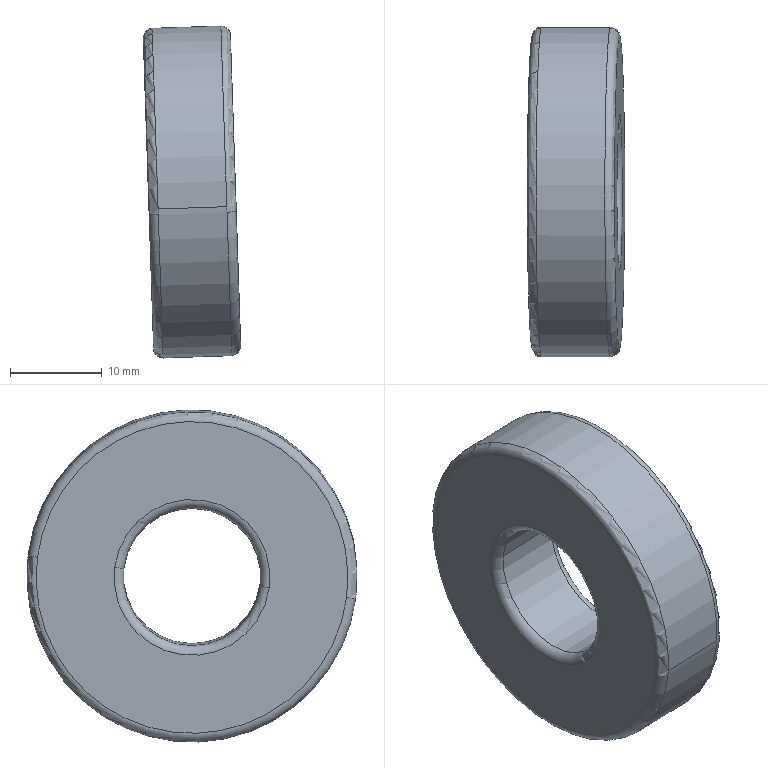Part | STEP file | 2026.6.15-Main Assembly图.sldasm-Part-94 | 1 solid | 14 faces | box 10.629 x 36.003 x 36.231 mm | volume 7922 mm3 | torus 8 | cylinder 4 | plane 2 | commonest cylinder face diameters 15 x2 36 x2
STEP:
#1=CARTESIAN_POINT('',(-1546.876,1321.722,3701.345));
#2=VERTEX_POINT('',#1);
#3=CARTESIAN_POINT('',(-1546.997,1357.487,3705.403));
#4=VERTEX_POINT('',#3);
#5=CARTESIAN_POINT('',(-1546.947,1339.57,3703.676));
#6=DIRECTION('',(0.9994,-0.0004028,0.03334));
#7=DIRECTION('',(-0.003921,0.9916,0.1295));
#8=AXIS2_PLACEMENT_3D('',#5,#6,#7);
#9=CIRCLE('',#8,18.);
#10=EDGE_CURVE('',#2,#4,#9,.T.);
#11=ORIENTED_EDGE('',*,*,#10,.F.);
#12=CARTESIAN_POINT('',(-1547.88,1322.714,3701.441));
#13=VERTEX_POINT('',#12);
#14=CARTESIAN_POINT('',(-1546.88,1322.713,3701.474));
#15=DIRECTION('',(0.03311,0.1296,-0.991));
#16=DIRECTION('',(0.,0.9916,0.1297));
#17=AXIS2_PLACEMENT_3D('',#14,#15,#16);
#18=CIRCLE('',#17,1.);
#19=EDGE_CURVE('',#2,#13,#18,.T.);
#20=ORIENTED_EDGE('',*,*,#19,.T.);
#21=CARTESIAN_POINT('',(-1548.013,1356.427,3705.845));
#22=VERTEX_POINT('',#21);
#23=CARTESIAN_POINT('',(-1547.946,1339.57,3703.643));
#24=DIRECTION('',(-0.9994,0.0004028,-0.03334));
#25=DIRECTION('',(-0.003921,0.9916,0.1295));
#26=AXIS2_PLACEMENT_3D('',#23,#24,#25);
#27=CIRCLE('',#26,17.);
#28=EDGE_CURVE('',#22,#13,#27,.T.);
#29=ORIENTED_EDGE('',*,*,#28,.F.);
#30=CARTESIAN_POINT('',(-1547.017,1357.418,3706.008));
#31=VERTEX_POINT('',#30);
#32=CARTESIAN_POINT('',(-1547.014,1356.427,3705.878));
#33=DIRECTION('',(-0.03311,-0.1296,0.991));
#34=DIRECTION('',(0.,-0.9916,-0.1297));
#35=AXIS2_PLACEMENT_3D('',#32,#33,#34);
#36=CIRCLE('',#35,1.);
#37=EDGE_CURVE('',#31,#22,#36,.T.);
#38=ORIENTED_EDGE('',*,*,#37,.F.);
#39=CARTESIAN_POINT('',(-1546.947,1339.57,3703.676));
#40=DIRECTION('',(0.9994,-0.0004028,0.03334));
#41=DIRECTION('',(-0.003921,0.9916,0.1295));
#42=AXIS2_PLACEMENT_3D('',#39,#40,#41);
#43=CIRCLE('',#42,18.);
#44=EDGE_CURVE('',#4,#31,#43,.T.);
#45=ORIENTED_EDGE('',*,*,#44,.F.);
#46=EDGE_LOOP('',(#11,#20,#29,#38,#45));
#47=FACE_OUTER_BOUND('',#46,.T.);
#48=CARTESIAN_POINT('',(-1546.947,1339.57,3703.676));
#49=DIRECTION('',(-0.9994,0.0004028,-0.03334));
#50=DIRECTION('',(-0.003921,0.9916,0.1295));
#51=AXIS2_PLACEMENT_3D('',#48,#49,#50);
#52=TOROIDAL_SURFACE('',#51,17.,1.);
#53=ADVANCED_FACE('',(#47),#52,.T.);
#54=CARTESIAN_POINT('',(-1547.913,1331.142,3702.542));
#55=VERTEX_POINT('',#54);
#56=CARTESIAN_POINT('',(-1547.98,1347.999,3704.744));
#57=VERTEX_POINT('',#56);
#58=CARTESIAN_POINT('',(-1547.946,1339.57,3703.643));
#59=DIRECTION('',(0.9994,-0.0004028,0.03334));
#60=DIRECTION('',(-0.003921,0.9916,0.1295));
#61=AXIS2_PLACEMENT_3D('',#58,#59,#60);
#62=CIRCLE('',#61,8.5);
#63=EDGE_CURVE('',#55,#57,#62,.T.);
#64=ORIENTED_EDGE('',*,*,#63,.F.);
#65=CARTESIAN_POINT('',(-1546.917,1332.133,3702.705));
#66=VERTEX_POINT('',#65);
#67=CARTESIAN_POINT('',(-1546.914,1331.142,3702.575));
#68=DIRECTION('',(0.03311,0.1296,-0.991));
#69=DIRECTION('',(0.,0.9916,0.1297));
#70=AXIS2_PLACEMENT_3D('',#67,#68,#69);
#71=CIRCLE('',#70,1.);
#72=EDGE_CURVE('',#55,#66,#71,.T.);
#73=ORIENTED_EDGE('',*,*,#72,.T.);
#74=CARTESIAN_POINT('',(-1546.976,1347.007,3704.648));
#75=VERTEX_POINT('',#74);
#76=CARTESIAN_POINT('',(-1546.947,1339.57,3703.676));
#77=DIRECTION('',(-0.9994,0.0004028,-0.03334));
#78=DIRECTION('',(-0.003921,0.9916,0.1295));
#79=AXIS2_PLACEMENT_3D('',#76,#77,#78);
#80=CIRCLE('',#79,7.5);
#81=EDGE_CURVE('',#75,#66,#80,.T.);
#82=ORIENTED_EDGE('',*,*,#81,.F.);
#83=CARTESIAN_POINT('',(-1546.98,1347.998,3704.777));
#84=DIRECTION('',(-0.03311,-0.1296,0.991));
#85=DIRECTION('',(0.,-0.9916,-0.1297));
#86=AXIS2_PLACEMENT_3D('',#83,#84,#85);
#87=CIRCLE('',#86,1.);
#88=EDGE_CURVE('',#57,#75,#87,.T.);
#89=ORIENTED_EDGE('',*,*,#88,.F.);
#90=EDGE_LOOP('',(#64,#73,#82,#89));
#91=FACE_OUTER_BOUND('',#90,.T.);
#92=CARTESIAN_POINT('',(-1546.947,1339.57,3703.676));
#93=DIRECTION('',(-0.9994,0.0004028,-0.03334));
#94=DIRECTION('',(-0.003921,0.9916,0.1295));
#95=AXIS2_PLACEMENT_3D('',#92,#93,#94);
#96=TOROIDAL_SURFACE('',#95,8.5,1.);
#97=ADVANCED_FACE('',(#91),#96,.T.);
#98=CARTESIAN_POINT('',(-1538.485,1347.995,3705.061));
#99=VERTEX_POINT('',#98);
#100=CARTESIAN_POINT('',(-1538.418,1331.138,3702.859));
#101=VERTEX_POINT('',#100);
#102=CARTESIAN_POINT('',(-1538.452,1339.567,3703.96));
#103=DIRECTION('',(-0.9994,0.0004028,-0.03334));
#104=DIRECTION('',(0.003921,-0.9916,-0.1295));
#105=AXIS2_PLACEMENT_3D('',#102,#103,#104);
#106=CIRCLE('',#105,8.5);
#107=EDGE_CURVE('',#99,#101,#106,.T.);
#108=ORIENTED_EDGE('',*,*,#107,.F.);
#109=CARTESIAN_POINT('',(-1539.48,1347.004,3704.898));
#110=VERTEX_POINT('',#109);
#111=CARTESIAN_POINT('',(-1539.484,1347.995,3705.027));
#112=DIRECTION('',(0.03311,0.1296,-0.991));
#113=DIRECTION('',(0.,0.9916,0.1297));
#114=AXIS2_PLACEMENT_3D('',#111,#112,#113);
#115=CIRCLE('',#114,1.);
#116=EDGE_CURVE('',#99,#110,#115,.T.);
#117=ORIENTED_EDGE('',*,*,#116,.T.);
#118=CARTESIAN_POINT('',(-1539.422,1332.13,3702.955));
#119=VERTEX_POINT('',#118);
#120=CARTESIAN_POINT('',(-1539.451,1339.567,3703.926));
#121=DIRECTION('',(0.9994,-0.0004028,0.03334));
#122=DIRECTION('',(0.003921,-0.9916,-0.1295));
#123=AXIS2_PLACEMENT_3D('',#120,#121,#122);
#124=CIRCLE('',#123,7.5);
#125=EDGE_CURVE('',#119,#110,#124,.T.);
#126=ORIENTED_EDGE('',*,*,#125,.F.);
#127=CARTESIAN_POINT('',(-1539.418,1331.139,3702.825));
#128=DIRECTION('',(-0.03311,-0.1296,0.991));
#129=DIRECTION('',(0.,-0.9916,-0.1297));
#130=AXIS2_PLACEMENT_3D('',#127,#128,#129);
#131=CIRCLE('',#130,1.);
#132=EDGE_CURVE('',#101,#119,#131,.T.);
#133=ORIENTED_EDGE('',*,*,#132,.F.);
#134=EDGE_LOOP('',(#108,#117,#126,#133));
#135=FACE_OUTER_BOUND('',#134,.T.);
#136=CARTESIAN_POINT('',(-1539.451,1339.567,3703.926));
#137=DIRECTION('',(0.9994,-0.0004028,0.03334));
#138=DIRECTION('',(0.003921,-0.9916,-0.1295));
#139=AXIS2_PLACEMENT_3D('',#136,#137,#138);
#140=TOROIDAL_SURFACE('',#139,8.5,1.);
#141=ADVANCED_FACE('',(#135),#140,.T.);
#142=CARTESIAN_POINT('',(-1539.522,1357.415,3706.258));
#143=VERTEX_POINT('',#142);
#144=CARTESIAN_POINT('',(-1539.501,1357.484,3705.653));
#145=VERTEX_POINT('',#144);
#146=CARTESIAN_POINT('',(-1539.451,1339.567,3703.926));
#147=DIRECTION('',(-0.9994,0.0004028,-0.03334));
#148=DIRECTION('',(0.003921,-0.9916,-0.1295));
#149=AXIS2_PLACEMENT_3D('',#146,#147,#148);
#150=CIRCLE('',#149,18.);
#151=EDGE_CURVE('',#143,#145,#150,.T.);
#152=ORIENTED_EDGE('',*,*,#151,.F.);
#153=CARTESIAN_POINT('',(-1538.518,1356.423,3706.162));
#154=VERTEX_POINT('',#153);
#155=CARTESIAN_POINT('',(-1539.518,1356.424,3706.128));
#156=DIRECTION('',(0.03311,0.1296,-0.991));
#157=DIRECTION('',(0.,0.9916,0.1297));
#158=AXIS2_PLACEMENT_3D('',#155,#156,#157);
#159=CIRCLE('',#158,1.);
#160=EDGE_CURVE('',#143,#154,#159,.T.);
#161=ORIENTED_EDGE('',*,*,#160,.T.);
#162=CARTESIAN_POINT('',(-1538.385,1322.71,3701.758));
#163=VERTEX_POINT('',#162);
#164=CARTESIAN_POINT('',(-1538.452,1339.567,3703.96));
#165=DIRECTION('',(0.9994,-0.0004028,0.03334));
#166=DIRECTION('',(0.003921,-0.9916,-0.1295));
#167=AXIS2_PLACEMENT_3D('',#164,#165,#166);
#168=CIRCLE('',#167,17.);
#169=EDGE_CURVE('',#163,#154,#168,.T.);
#170=ORIENTED_EDGE('',*,*,#169,.F.);
#171=CARTESIAN_POINT('',(-1539.38,1321.719,3701.595));
#172=VERTEX_POINT('',#171);
#173=CARTESIAN_POINT('',(-1539.384,1322.71,3701.724));
#174=DIRECTION('',(-0.03311,-0.1296,0.991));
#175=DIRECTION('',(0.,-0.9916,-0.1297));
#176=AXIS2_PLACEMENT_3D('',#173,#174,#175);
#177=CIRCLE('',#176,1.);
#178=EDGE_CURVE('',#172,#163,#177,.T.);
#179=ORIENTED_EDGE('',*,*,#178,.F.);
#180=CARTESIAN_POINT('',(-1539.451,1339.567,3703.926));
#181=DIRECTION('',(-0.9994,0.0004028,-0.03334));
#182=DIRECTION('',(0.003921,-0.9916,-0.1295));
#183=AXIS2_PLACEMENT_3D('',#180,#181,#182);
#184=CIRCLE('',#183,18.);
#185=EDGE_CURVE('',#145,#172,#184,.T.);
#186=ORIENTED_EDGE('',*,*,#185,.F.);
#187=EDGE_LOOP('',(#152,#161,#170,#179,#186));
#188=FACE_OUTER_BOUND('',#187,.T.);
#189=CARTESIAN_POINT('',(-1539.451,1339.567,3703.926));
#190=DIRECTION('',(0.9994,-0.0004028,0.03334));
#191=DIRECTION('',(0.003921,-0.9916,-0.1295));
#192=AXIS2_PLACEMENT_3D('',#189,#190,#191);
#193=TOROIDAL_SURFACE('',#192,17.,1.);
#194=ADVANCED_FACE('',(#188),#193,.T.);
#195=CARTESIAN_POINT('',(-1546.947,1339.57,3703.676));
#196=DIRECTION('',(-0.9994,0.0004028,-0.03334));
#197=DIRECTION('',(-0.003921,0.9916,0.1295));
#198=AXIS2_PLACEMENT_3D('',#195,#196,#197);
#199=CIRCLE('',#198,7.5);
#200=EDGE_CURVE('',#66,#75,#199,.T.);
#201=ORIENTED_EDGE('',*,*,#200,.T.);
#202=CARTESIAN_POINT('',(-1547.976,1347.007,3704.614));
#203=DIRECTION('',(0.9994,-0.0004028,0.03334));
#204=VECTOR('',#203,1000.);
#205=LINE('',#202,#204);
#206=EDGE_CURVE('',#75,#110,#205,.T.);
#207=ORIENTED_EDGE('',*,*,#206,.T.);
#208=CARTESIAN_POINT('',(-1539.451,1339.567,3703.926));
#209=DIRECTION('',(0.9994,-0.0004028,0.03334));
#210=DIRECTION('',(0.003921,-0.9916,-0.1295));
#211=AXIS2_PLACEMENT_3D('',#208,#209,#210);
#212=CIRCLE('',#211,7.5);
#213=EDGE_CURVE('',#110,#119,#212,.T.);
#214=ORIENTED_EDGE('',*,*,#213,.T.);
#215=CARTESIAN_POINT('',(-1547.917,1332.134,3702.671));
#216=DIRECTION('',(0.9994,-0.0004028,0.03334));
#217=VECTOR('',#216,1000.);
#218=LINE('',#215,#217);
#219=EDGE_CURVE('',#66,#119,#218,.T.);
#220=ORIENTED_EDGE('',*,*,#219,.F.);
#221=EDGE_LOOP('',(#201,#207,#214,#220));
#222=FACE_OUTER_BOUND('',#221,.T.);
#223=CARTESIAN_POINT('',(-1547.946,1339.57,3703.643));
#224=DIRECTION('',(0.9994,-0.0004028,0.03334));
#225=DIRECTION('',(0.003921,-0.9916,-0.1295));
#226=AXIS2_PLACEMENT_3D('',#223,#224,#225);
#227=CYLINDRICAL_SURFACE('',#226,7.5);
#228=ADVANCED_FACE('',(#222),#227,.F.);
#229=ORIENTED_EDGE('',*,*,#44,.T.);
#230=CARTESIAN_POINT('',(-1546.896,1321.653,3701.949));
#231=VERTEX_POINT('',#230);
#232=CARTESIAN_POINT('',(-1546.947,1339.57,3703.676));
#233=DIRECTION('',(0.9994,-0.0004028,0.03334));
#234=DIRECTION('',(-0.003921,0.9916,0.1295));
#235=AXIS2_PLACEMENT_3D('',#232,#233,#234);
#236=CIRCLE('',#235,18.);
#237=EDGE_CURVE('',#31,#231,#236,.T.);
#238=ORIENTED_EDGE('',*,*,#237,.T.);
#239=CARTESIAN_POINT('',(-1539.401,1321.65,3702.199));
#240=VERTEX_POINT('',#239);
#241=CARTESIAN_POINT('',(-1547.896,1321.653,3701.916));
#242=DIRECTION('',(0.9994,-0.0004028,0.03334));
#243=VECTOR('',#242,1000.);
#244=LINE('',#241,#243);
#245=EDGE_CURVE('',#231,#240,#244,.T.);
#246=ORIENTED_EDGE('',*,*,#245,.T.);
#247=CARTESIAN_POINT('',(-1539.451,1339.567,3703.926));
#248=DIRECTION('',(-0.9994,0.0004028,-0.03334));
#249=DIRECTION('',(0.003921,-0.9916,-0.1295));
#250=AXIS2_PLACEMENT_3D('',#247,#248,#249);
#251=CIRCLE('',#250,18.);
#252=EDGE_CURVE('',#240,#143,#251,.T.);
#253=ORIENTED_EDGE('',*,*,#252,.T.);
#254=ORIENTED_EDGE('',*,*,#151,.T.);
#255=CARTESIAN_POINT('',(-1547.997,1357.487,3705.37));
#256=DIRECTION('',(0.9994,-0.0004028,0.03334));
#257=VECTOR('',#256,1000.);
#258=LINE('',#255,#257);
#259=EDGE_CURVE('',#4,#145,#258,.T.);
#260=ORIENTED_EDGE('',*,*,#259,.F.);
#261=EDGE_LOOP('',(#229,#238,#246,#253,#254,#260));
#262=FACE_OUTER_BOUND('',#261,.T.);
#263=CARTESIAN_POINT('',(-1547.946,1339.57,3703.643));
#264=DIRECTION('',(0.9994,-0.0004028,0.03334));
#265=DIRECTION('',(-0.002799,0.9954,0.09594));
#266=AXIS2_PLACEMENT_3D('',#263,#264,#265);
#267=CYLINDRICAL_SURFACE('',#266,18.);
#268=ADVANCED_FACE('',(#262),#267,.T.);
#269=ORIENTED_EDGE('',*,*,#169,.T.);
#270=CARTESIAN_POINT('',(-1538.452,1339.567,3703.96));
#271=DIRECTION('',(0.9994,-0.0004028,0.03334));
#272=DIRECTION('',(0.003921,-0.9916,-0.1295));
#273=AXIS2_PLACEMENT_3D('',#270,#271,#272);
#274=CIRCLE('',#273,17.);
#275=EDGE_CURVE('',#154,#163,#274,.T.);
#276=ORIENTED_EDGE('',*,*,#275,.T.);
#277=EDGE_LOOP('',(#269,#276));
#278=FACE_OUTER_BOUND('',#277,.T.);
#279=CARTESIAN_POINT('',(-1538.452,1339.567,3703.96));
#280=DIRECTION('',(-0.9994,0.0004028,-0.03334));
#281=DIRECTION('',(0.003921,-0.9916,-0.1295));
#282=AXIS2_PLACEMENT_3D('',#279,#280,#281);
#283=CIRCLE('',#282,8.5);
#284=EDGE_CURVE('',#101,#99,#283,.T.);
#285=ORIENTED_EDGE('',*,*,#284,.T.);
#286=ORIENTED_EDGE('',*,*,#107,.T.);
#287=EDGE_LOOP('',(#285,#286));
#288=FACE_BOUND('',#287,.T.);
#289=CARTESIAN_POINT('',(-1538.452,1339.567,3703.96));
#290=DIRECTION('',(0.9994,-0.0004028,0.03334));
#291=DIRECTION('',(0.003921,-0.9916,-0.1295));
#292=AXIS2_PLACEMENT_3D('',#289,#290,#291);
#293=PLANE('',#292);
#294=ADVANCED_FACE('',(#278,#288),#293,.T.);
#295=CARTESIAN_POINT('',(-1547.946,1339.57,3703.643));
#296=DIRECTION('',(0.9994,-0.0004028,0.03334));
#297=DIRECTION('',(-0.003921,0.9916,0.1295));
#298=AXIS2_PLACEMENT_3D('',#295,#296,#297);
#299=CIRCLE('',#298,8.5);
#300=EDGE_CURVE('',#57,#55,#299,.T.);
#301=ORIENTED_EDGE('',*,*,#300,.T.);
#302=ORIENTED_EDGE('',*,*,#63,.T.);
#303=EDGE_LOOP('',(#301,#302));
#304=FACE_BOUND('',#303,.T.);
#305=ORIENTED_EDGE('',*,*,#28,.T.);
#306=CARTESIAN_POINT('',(-1547.946,1339.57,3703.643));
#307=DIRECTION('',(-0.9994,0.0004028,-0.03334));
#308=DIRECTION('',(-0.003921,0.9916,0.1295));
#309=AXIS2_PLACEMENT_3D('',#306,#307,#308);
#310=CIRCLE('',#309,17.);
#311=EDGE_CURVE('',#13,#22,#310,.T.);
#312=ORIENTED_EDGE('',*,*,#311,.T.);
#313=EDGE_LOOP('',(#305,#312));
#314=FACE_OUTER_BOUND('',#313,.T.);
#315=CARTESIAN_POINT('',(-1547.946,1339.57,3703.643));
#316=DIRECTION('',(-0.9994,0.0004028,-0.03334));
#317=DIRECTION('',(-0.003921,0.9916,0.1295));
#318=AXIS2_PLACEMENT_3D('',#315,#316,#317);
#319=PLANE('',#318);
#320=ADVANCED_FACE('',(#304,#314),#319,.T.);
#321=ORIENTED_EDGE('',*,*,#245,.F.);
#322=CARTESIAN_POINT('',(-1546.947,1339.57,3703.676));
#323=DIRECTION('',(0.9994,-0.0004028,0.03334));
#324=DIRECTION('',(-0.003921,0.9916,0.1295));
#325=AXIS2_PLACEMENT_3D('',#322,#323,#324);
#326=CIRCLE('',#325,18.);
#327=EDGE_CURVE('',#231,#2,#326,.T.);
#328=ORIENTED_EDGE('',*,*,#327,.T.);
#329=ORIENTED_EDGE('',*,*,#10,.T.);
#330=ORIENTED_EDGE('',*,*,#259,.T.);
#331=ORIENTED_EDGE('',*,*,#185,.T.);
#332=CARTESIAN_POINT('',(-1539.451,1339.567,3703.926));
#333=DIRECTION('',(-0.9994,0.0004028,-0.03334));
#334=DIRECTION('',(0.003921,-0.9916,-0.1295));
#335=AXIS2_PLACEMENT_3D('',#332,#333,#334);
#336=CIRCLE('',#335,18.);
#337=EDGE_CURVE('',#172,#240,#336,.T.);
#338=ORIENTED_EDGE('',*,*,#337,.T.);
#339=EDGE_LOOP('',(#321,#328,#329,#330,#331,#338));
#340=FACE_OUTER_BOUND('',#339,.T.);
#341=CARTESIAN_POINT('',(-1547.946,1339.57,3703.643));
#342=DIRECTION('',(0.9994,-0.0004028,0.03334));
#343=DIRECTION('',(-0.002799,0.9954,0.09594));
#344=AXIS2_PLACEMENT_3D('',#341,#342,#343);
#345=CYLINDRICAL_SURFACE('',#344,18.);
#346=ADVANCED_FACE('',(#340),#345,.T.);
#347=ORIENTED_EDGE('',*,*,#206,.F.);
#348=ORIENTED_EDGE('',*,*,#81,.T.);
#349=ORIENTED_EDGE('',*,*,#219,.T.);
#350=ORIENTED_EDGE('',*,*,#125,.T.);
#351=EDGE_LOOP('',(#347,#348,#349,#350));
#352=FACE_OUTER_BOUND('',#351,.T.);
#353=CARTESIAN_POINT('',(-1547.946,1339.57,3703.643));
#354=DIRECTION('',(0.9994,-0.0004028,0.03334));
#355=DIRECTION('',(0.003921,-0.9916,-0.1295));
#356=AXIS2_PLACEMENT_3D('',#353,#354,#355);
#357=CYLINDRICAL_SURFACE('',#356,7.5);
#358=ADVANCED_FACE('',(#352),#357,.F.);
#359=ORIENTED_EDGE('',*,*,#160,.F.);
#360=ORIENTED_EDGE('',*,*,#252,.F.);
#361=ORIENTED_EDGE('',*,*,#337,.F.);
#362=ORIENTED_EDGE('',*,*,#178,.T.);
#363=ORIENTED_EDGE('',*,*,#275,.F.);
#364=EDGE_LOOP('',(#359,#360,#361,#362,#363));
#365=FACE_OUTER_BOUND('',#364,.T.);
#366=CARTESIAN_POINT('',(-1539.451,1339.567,3703.926));
#367=DIRECTION('',(0.9994,-0.0004028,0.03334));
#368=DIRECTION('',(0.003921,-0.9916,-0.1295));
#369=AXIS2_PLACEMENT_3D('',#366,#367,#368);
#370=TOROIDAL_SURFACE('',#369,17.,1.);
#371=ADVANCED_FACE('',(#365),#370,.T.);
#372=ORIENTED_EDGE('',*,*,#116,.F.);
#373=ORIENTED_EDGE('',*,*,#284,.F.);
#374=ORIENTED_EDGE('',*,*,#132,.T.);
#375=ORIENTED_EDGE('',*,*,#213,.F.);
#376=EDGE_LOOP('',(#372,#373,#374,#375));
#377=FACE_OUTER_BOUND('',#376,.T.);
#378=CARTESIAN_POINT('',(-1539.451,1339.567,3703.926));
#379=DIRECTION('',(0.9994,-0.0004028,0.03334));
#380=DIRECTION('',(0.003921,-0.9916,-0.1295));
#381=AXIS2_PLACEMENT_3D('',#378,#379,#380);
#382=TOROIDAL_SURFACE('',#381,8.5,1.);
#383=ADVANCED_FACE('',(#377),#382,.T.);
#384=ORIENTED_EDGE('',*,*,#72,.F.);
#385=ORIENTED_EDGE('',*,*,#300,.F.);
#386=ORIENTED_EDGE('',*,*,#88,.T.);
#387=ORIENTED_EDGE('',*,*,#200,.F.);
#388=EDGE_LOOP('',(#384,#385,#386,#387));
#389=FACE_OUTER_BOUND('',#388,.T.);
#390=CARTESIAN_POINT('',(-1546.947,1339.57,3703.676));
#391=DIRECTION('',(-0.9994,0.0004028,-0.03334));
#392=DIRECTION('',(-0.003921,0.9916,0.1295));
#393=AXIS2_PLACEMENT_3D('',#390,#391,#392);
#394=TOROIDAL_SURFACE('',#393,8.5,1.);
#395=ADVANCED_FACE('',(#389),#394,.T.);
#396=ORIENTED_EDGE('',*,*,#19,.F.);
#397=ORIENTED_EDGE('',*,*,#327,.F.);
#398=ORIENTED_EDGE('',*,*,#237,.F.);
#399=ORIENTED_EDGE('',*,*,#37,.T.);
#400=ORIENTED_EDGE('',*,*,#311,.F.);
#401=EDGE_LOOP('',(#396,#397,#398,#399,#400));
#402=FACE_OUTER_BOUND('',#401,.T.);
#403=CARTESIAN_POINT('',(-1546.947,1339.57,3703.676));
#404=DIRECTION('',(-0.9994,0.0004028,-0.03334));
#405=DIRECTION('',(-0.003921,0.9916,0.1295));
#406=AXIS2_PLACEMENT_3D('',#403,#404,#405);
#407=TOROIDAL_SURFACE('',#406,17.,1.);
#408=ADVANCED_FACE('',(#402),#407,.T.);
#409=CLOSED_SHELL('',(#53,#97,#141,#194,#228,#268,#294,#320,#346,#358,#371,#383,#395,#408));
#410=MANIFOLD_SOLID_BREP('',#409);
#411=CARTESIAN_POINT('',(0.,0.,0.));
#412=DIRECTION('',(0.,0.,1.));
#413=DIRECTION('',(1.,0.,0.));
#414=AXIS2_PLACEMENT_3D('',#411,#412,#413);
#415=(LENGTH_UNIT()NAMED_UNIT(*)SI_UNIT(.MILLI.,.METRE.));
#416=UNCERTAINTY_MEASURE_WITH_UNIT(LENGTH_MEASURE(0.00001),#415,'','');
#417=(NAMED_UNIT(*)PLANE_ANGLE_UNIT()SI_UNIT($,.RADIAN.));
#418=(NAMED_UNIT(*)SI_UNIT($,.STERADIAN.)SOLID_ANGLE_UNIT());
#419=(GEOMETRIC_REPRESENTATION_CONTEXT(3)GLOBAL_UNCERTAINTY_ASSIGNED_CONTEXT((#416))GLOBAL_UNIT_ASSIGNED_CONTEXT((#415,#417,#418))REPRESENTATION_CONTEXT('',''));
#420=ADVANCED_BREP_SHAPE_REPRESENTATION('',(#410,#414),#419);